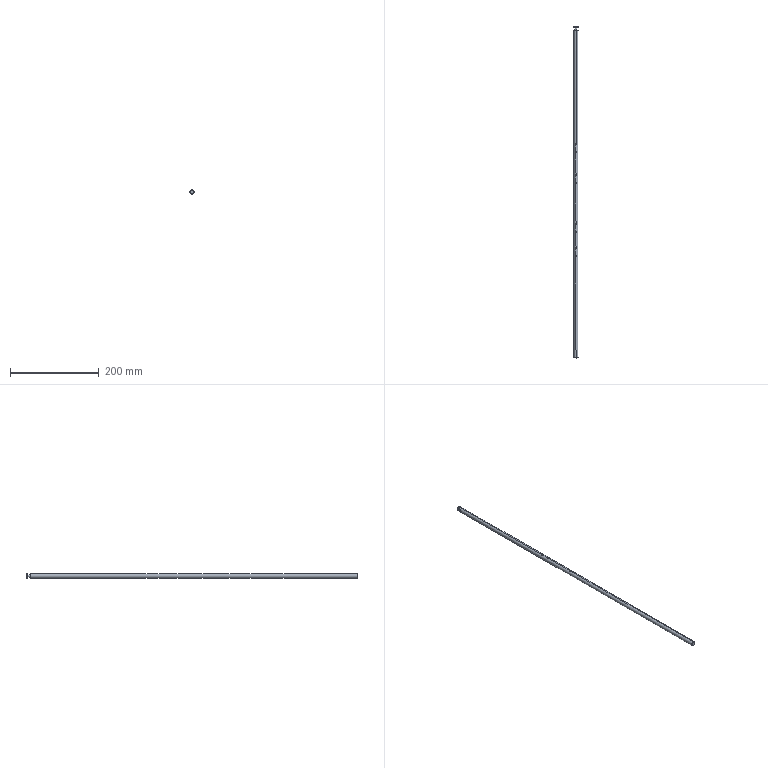Part | STEP file | 8XS234011 | 1 solid | 28 faces | box 10 x 750 x 10 mm | volume 58101 mm3 | cylinder 22 | plane 4 | cone 2 | commonest cylinder face diameters 2.8 x16 10 x4 6 x2